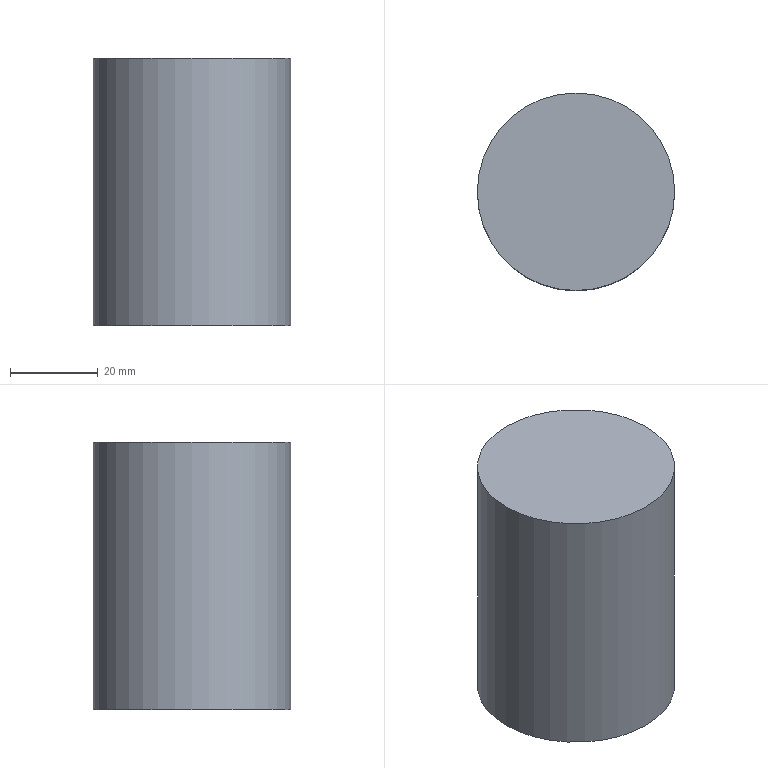Part | NX | features solid 2 | 1 solid | 3 faces | box 45 x 45 x 61 mm | volume 97016 mm3 | plane 2 | cylinder 1 | commonest cylinder face diameters 45 x1
STEP:
#1=CARTESIAN_POINT('',(1317.5,-830.,-45.));
#2=VERTEX_POINT('',#1);
#3=CARTESIAN_POINT('',(1295.,-830.,-45.));
#4=DIRECTION('',(0.,0.,1.));
#5=DIRECTION('',(1.,0.,0.));
#6=AXIS2_PLACEMENT_3D('',#3,#4,#5);
#7=CIRCLE('',#6,22.5);
#8=EDGE_CURVE('',#2,#2,#7,.F.);
#9=ORIENTED_EDGE('',*,*,#8,.F.);
#10=EDGE_LOOP('',(#9));
#11=FACE_BOUND('',#10,.T.);
#12=CARTESIAN_POINT('',(1272.5,-830.,16.));
#13=VERTEX_POINT('',#12);
#14=CARTESIAN_POINT('',(1295.,-830.,16.));
#15=DIRECTION('',(0.,0.,-1.));
#16=DIRECTION('',(-1.,0.,0.));
#17=AXIS2_PLACEMENT_3D('',#14,#15,#16);
#18=CIRCLE('',#17,22.5);
#19=EDGE_CURVE('',#13,#13,#18,.T.);
#20=ORIENTED_EDGE('',*,*,#19,.T.);
#21=EDGE_LOOP('',(#20));
#22=FACE_BOUND('',#21,.T.);
#23=CARTESIAN_POINT('',(1295.,-830.,-53.));
#24=DIRECTION('',(0.,0.,1.));
#25=DIRECTION('',(1.,0.,0.));
#26=AXIS2_PLACEMENT_3D('',#23,#24,#25);
#27=CYLINDRICAL_SURFACE('',#26,22.5);
#28=ADVANCED_FACE('',(#11,#22),#27,.T.);
#29=ORIENTED_EDGE('',*,*,#8,.T.);
#30=EDGE_LOOP('',(#29));
#31=FACE_BOUND('',#30,.T.);
#32=CARTESIAN_POINT('',(1295.,-838.25,-45.));
#33=DIRECTION('',(0.,0.,1.));
#34=DIRECTION('',(-1.,0.,0.));
#35=AXIS2_PLACEMENT_3D('',#32,#33,#34);
#36=PLANE('',#35);
#37=ADVANCED_FACE('',(#31),#36,.F.);
#38=ORIENTED_EDGE('',*,*,#19,.F.);
#39=EDGE_LOOP('',(#38));
#40=FACE_BOUND('',#39,.T.);
#41=CARTESIAN_POINT('',(1295.,-838.25,16.));
#42=DIRECTION('',(0.,0.,1.));
#43=DIRECTION('',(-1.,0.,0.));
#44=AXIS2_PLACEMENT_3D('',#41,#42,#43);
#45=PLANE('',#44);
#46=ADVANCED_FACE('',(#40),#45,.T.);
#47=CLOSED_SHELL('',(#28,#37,#46));
#48=MANIFOLD_SOLID_BREP('',#47);
#49=(LENGTH_UNIT()NAMED_UNIT(*)SI_UNIT(.MILLI.,.METRE.));
#50=UNCERTAINTY_MEASURE_WITH_UNIT(LENGTH_MEASURE(0.00001),#49,'','');
#51=(NAMED_UNIT(*)PLANE_ANGLE_UNIT()SI_UNIT($,.RADIAN.));
#52=(NAMED_UNIT(*)SI_UNIT($,.STERADIAN.)SOLID_ANGLE_UNIT());
#53=(GEOMETRIC_REPRESENTATION_CONTEXT(3)GLOBAL_UNCERTAINTY_ASSIGNED_CONTEXT((#50))GLOBAL_UNIT_ASSIGNED_CONTEXT((#49,#51,#52))REPRESENTATION_CONTEXT('',''));
#54=ADVANCED_BREP_SHAPE_REPRESENTATION('',(#48),#53);